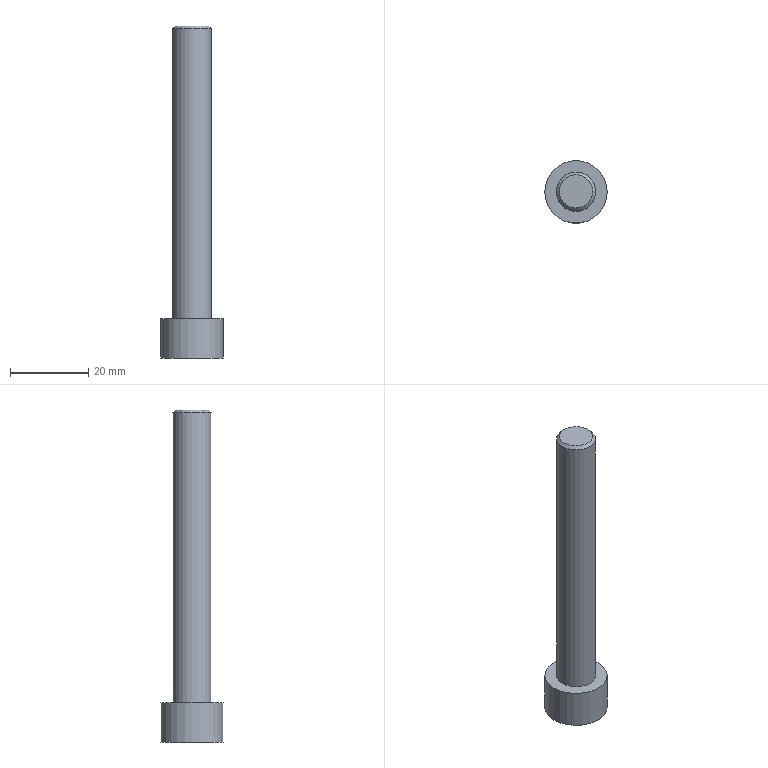Part | STEP file | gslz 2016.10.28-6_id290_x_t | 1 solid | 13 faces | box 16 x 16 x 85 mm | volume 7560 mm3 | plane 10 | cylinder 2 | cone 1 | commonest cylinder face diameters 10 x1 16 x1
STEP:
#1=CARTESIAN_POINT('',(-19.95,98.309,66.992));
#2=VERTEX_POINT('',#1);
#3=CARTESIAN_POINT('',(-19.95,93.691,66.992));
#4=VERTEX_POINT('',#3);
#5=CARTESIAN_POINT('',(-19.95,98.309,66.992));
#6=DIRECTION('',(0.,-1.,0.));
#7=VECTOR('',#6,1.);
#8=LINE('',#5,#7);
#9=EDGE_CURVE('',#2,#4,#8,.T.);
#10=ORIENTED_EDGE('',*,*,#9,.T.);
#11=CARTESIAN_POINT('',(-15.95,91.381,66.992));
#12=VERTEX_POINT('',#11);
#13=CARTESIAN_POINT('',(-19.95,93.691,66.992));
#14=DIRECTION('',(0.866,-0.5,0.));
#15=VECTOR('',#14,1.);
#16=LINE('',#13,#15);
#17=EDGE_CURVE('',#4,#12,#16,.T.);
#18=ORIENTED_EDGE('',*,*,#17,.T.);
#19=CARTESIAN_POINT('',(-11.95,93.691,66.992));
#20=VERTEX_POINT('',#19);
#21=CARTESIAN_POINT('',(-15.95,91.381,66.992));
#22=DIRECTION('',(0.866,0.5,0.));
#23=VECTOR('',#22,1.);
#24=LINE('',#21,#23);
#25=EDGE_CURVE('',#12,#20,#24,.T.);
#26=ORIENTED_EDGE('',*,*,#25,.T.);
#27=CARTESIAN_POINT('',(-11.95,98.309,66.992));
#28=VERTEX_POINT('',#27);
#29=CARTESIAN_POINT('',(-11.95,93.691,66.992));
#30=DIRECTION('',(0.,1.,0.));
#31=VECTOR('',#30,1.);
#32=LINE('',#29,#31);
#33=EDGE_CURVE('',#20,#28,#32,.T.);
#34=ORIENTED_EDGE('',*,*,#33,.T.);
#35=CARTESIAN_POINT('',(-15.95,100.619,66.992));
#36=VERTEX_POINT('',#35);
#37=CARTESIAN_POINT('',(-11.95,98.309,66.992));
#38=DIRECTION('',(-0.866,0.5,0.));
#39=VECTOR('',#38,1.);
#40=LINE('',#37,#39);
#41=EDGE_CURVE('',#28,#36,#40,.T.);
#42=ORIENTED_EDGE('',*,*,#41,.T.);
#43=CARTESIAN_POINT('',(-15.95,100.619,66.992));
#44=DIRECTION('',(-0.866,-0.5,0.));
#45=VECTOR('',#44,1.);
#46=LINE('',#43,#45);
#47=EDGE_CURVE('',#36,#2,#46,.T.);
#48=ORIENTED_EDGE('',*,*,#47,.T.);
#49=EDGE_LOOP('',(#10,#18,#26,#34,#42,#48));
#50=FACE_BOUND('',#49,.T.);
#51=CARTESIAN_POINT('',(-7.95,96.,66.992));
#52=VERTEX_POINT('',#51);
#53=CARTESIAN_POINT('',(-15.95,96.,66.992));
#54=DIRECTION('',(0.,0.,-1.));
#55=DIRECTION('',(1.,0.,0.));
#56=AXIS2_PLACEMENT_3D('',#53,#54,#55);
#57=CIRCLE('',#56,8.);
#58=EDGE_CURVE('',#52,#52,#57,.T.);
#59=ORIENTED_EDGE('',*,*,#58,.T.);
#60=EDGE_LOOP('',(#59));
#61=FACE_BOUND('',#60,.T.);
#62=CARTESIAN_POINT('',(-15.95,96.,66.992));
#63=DIRECTION('',(0.,0.,-1.));
#64=DIRECTION('',(-1.,0.,0.));
#65=AXIS2_PLACEMENT_3D('',#62,#63,#64);
#66=PLANE('',#65);
#67=ADVANCED_FACE('',(#50,#61),#66,.T.);
#68=CARTESIAN_POINT('',(-20.2,96.,151.992));
#69=VERTEX_POINT('',#68);
#70=CARTESIAN_POINT('',(-15.95,96.,151.992));
#71=DIRECTION('',(0.,0.,-1.));
#72=DIRECTION('',(-1.,0.,0.));
#73=AXIS2_PLACEMENT_3D('',#70,#71,#72);
#74=CIRCLE('',#73,4.25);
#75=EDGE_CURVE('',#69,#69,#74,.T.);
#76=ORIENTED_EDGE('',*,*,#75,.F.);
#77=EDGE_LOOP('',(#76));
#78=FACE_OUTER_BOUND('',#77,.T.);
#79=CARTESIAN_POINT('',(-15.95,96.,151.992));
#80=DIRECTION('',(0.,0.,1.));
#81=DIRECTION('',(1.,0.,0.));
#82=AXIS2_PLACEMENT_3D('',#79,#80,#81);
#83=PLANE('',#82);
#84=ADVANCED_FACE('',(#78),#83,.T.);
#85=CARTESIAN_POINT('',(-20.95,96.,151.242));
#86=VERTEX_POINT('',#85);
#87=CARTESIAN_POINT('',(-15.95,96.,151.242));
#88=DIRECTION('',(0.,0.,1.));
#89=DIRECTION('',(-1.,0.,0.));
#90=AXIS2_PLACEMENT_3D('',#87,#88,#89);
#91=CIRCLE('',#90,5.);
#92=EDGE_CURVE('',#86,#86,#91,.T.);
#93=ORIENTED_EDGE('',*,*,#92,.F.);
#94=EDGE_LOOP('',(#93));
#95=FACE_BOUND('',#94,.T.);
#96=CARTESIAN_POINT('',(-20.95,96.,76.992));
#97=VERTEX_POINT('',#96);
#98=CARTESIAN_POINT('',(-15.95,96.,76.992));
#99=DIRECTION('',(0.,0.,-1.));
#100=DIRECTION('',(-1.,0.,0.));
#101=AXIS2_PLACEMENT_3D('',#98,#99,#100);
#102=CIRCLE('',#101,5.);
#103=EDGE_CURVE('',#97,#97,#102,.T.);
#104=ORIENTED_EDGE('',*,*,#103,.F.);
#105=EDGE_LOOP('',(#104));
#106=FACE_BOUND('',#105,.T.);
#107=CARTESIAN_POINT('',(-15.95,96.,96.992));
#108=DIRECTION('',(0.,0.,1.));
#109=DIRECTION('',(1.,0.,0.));
#110=AXIS2_PLACEMENT_3D('',#107,#108,#109);
#111=CYLINDRICAL_SURFACE('',#110,5.);
#112=ADVANCED_FACE('',(#95,#106),#111,.T.);
#113=ORIENTED_EDGE('',*,*,#103,.T.);
#114=EDGE_LOOP('',(#113));
#115=FACE_BOUND('',#114,.T.);
#116=CARTESIAN_POINT('',(-23.95,96.,76.992));
#117=VERTEX_POINT('',#116);
#118=CARTESIAN_POINT('',(-15.95,96.,76.992));
#119=DIRECTION('',(0.,0.,-1.));
#120=DIRECTION('',(-1.,0.,0.));
#121=AXIS2_PLACEMENT_3D('',#118,#119,#120);
#122=CIRCLE('',#121,8.);
#123=EDGE_CURVE('',#117,#117,#122,.T.);
#124=ORIENTED_EDGE('',*,*,#123,.F.);
#125=EDGE_LOOP('',(#124));
#126=FACE_BOUND('',#125,.T.);
#127=CARTESIAN_POINT('',(-15.95,96.,76.992));
#128=DIRECTION('',(0.,0.,1.));
#129=DIRECTION('',(1.,0.,0.));
#130=AXIS2_PLACEMENT_3D('',#127,#128,#129);
#131=PLANE('',#130);
#132=ADVANCED_FACE('',(#115,#126),#131,.T.);
#133=ORIENTED_EDGE('',*,*,#123,.T.);
#134=EDGE_LOOP('',(#133));
#135=FACE_BOUND('',#134,.T.);
#136=ORIENTED_EDGE('',*,*,#58,.F.);
#137=EDGE_LOOP('',(#136));
#138=FACE_BOUND('',#137,.T.);
#139=CARTESIAN_POINT('',(-15.95,96.,63.992));
#140=DIRECTION('',(0.,0.,1.));
#141=DIRECTION('',(1.,0.,0.));
#142=AXIS2_PLACEMENT_3D('',#139,#140,#141);
#143=CYLINDRICAL_SURFACE('',#142,8.);
#144=ADVANCED_FACE('',(#135,#138),#143,.T.);
#145=ORIENTED_EDGE('',*,*,#9,.F.);
#146=CARTESIAN_POINT('',(-19.95,98.309,72.992));
#147=VERTEX_POINT('',#146);
#148=CARTESIAN_POINT('',(-19.95,98.309,72.992));
#149=DIRECTION('',(0.,0.,1.));
#150=VECTOR('',#149,1.);
#151=LINE('',#148,#150);
#152=EDGE_CURVE('',#2,#147,#151,.T.);
#153=ORIENTED_EDGE('',*,*,#152,.T.);
#154=CARTESIAN_POINT('',(-19.95,93.691,72.992));
#155=VERTEX_POINT('',#154);
#156=CARTESIAN_POINT('',(-19.95,98.309,72.992));
#157=DIRECTION('',(0.,1.,0.));
#158=VECTOR('',#157,1.);
#159=LINE('',#156,#158);
#160=EDGE_CURVE('',#155,#147,#159,.T.);
#161=ORIENTED_EDGE('',*,*,#160,.F.);
#162=CARTESIAN_POINT('',(-19.95,93.691,72.992));
#163=DIRECTION('',(0.,0.,1.));
#164=VECTOR('',#163,1.);
#165=LINE('',#162,#164);
#166=EDGE_CURVE('',#4,#155,#165,.T.);
#167=ORIENTED_EDGE('',*,*,#166,.F.);
#168=EDGE_LOOP('',(#145,#153,#161,#167));
#169=FACE_OUTER_BOUND('',#168,.T.);
#170=CARTESIAN_POINT('',(-19.95,98.309,72.992));
#171=DIRECTION('',(-1.,0.,0.));
#172=DIRECTION('',(0.,0.,1.));
#173=AXIS2_PLACEMENT_3D('',#170,#171,#172);
#174=PLANE('',#173);
#175=ADVANCED_FACE('',(#169),#174,.F.);
#176=ORIENTED_EDGE('',*,*,#17,.F.);
#177=ORIENTED_EDGE('',*,*,#166,.T.);
#178=CARTESIAN_POINT('',(-15.95,91.381,72.992));
#179=VERTEX_POINT('',#178);
#180=CARTESIAN_POINT('',(-19.95,93.691,72.992));
#181=DIRECTION('',(-0.866,0.5,0.));
#182=VECTOR('',#181,1.);
#183=LINE('',#180,#182);
#184=EDGE_CURVE('',#179,#155,#183,.T.);
#185=ORIENTED_EDGE('',*,*,#184,.F.);
#186=CARTESIAN_POINT('',(-15.95,91.381,72.992));
#187=DIRECTION('',(0.,0.,1.));
#188=VECTOR('',#187,1.);
#189=LINE('',#186,#188);
#190=EDGE_CURVE('',#12,#179,#189,.T.);
#191=ORIENTED_EDGE('',*,*,#190,.F.);
#192=EDGE_LOOP('',(#176,#177,#185,#191));
#193=FACE_OUTER_BOUND('',#192,.T.);
#194=CARTESIAN_POINT('',(-19.95,93.691,72.992));
#195=DIRECTION('',(-0.5,-0.866,0.));
#196=DIRECTION('',(-0.866,0.5,0.));
#197=AXIS2_PLACEMENT_3D('',#194,#195,#196);
#198=PLANE('',#197);
#199=ADVANCED_FACE('',(#193),#198,.F.);
#200=ORIENTED_EDGE('',*,*,#25,.F.);
#201=ORIENTED_EDGE('',*,*,#190,.T.);
#202=CARTESIAN_POINT('',(-11.95,93.691,72.992));
#203=VERTEX_POINT('',#202);
#204=CARTESIAN_POINT('',(-15.95,91.381,72.992));
#205=DIRECTION('',(-0.866,-0.5,0.));
#206=VECTOR('',#205,1.);
#207=LINE('',#204,#206);
#208=EDGE_CURVE('',#203,#179,#207,.T.);
#209=ORIENTED_EDGE('',*,*,#208,.F.);
#210=CARTESIAN_POINT('',(-11.95,93.691,72.992));
#211=DIRECTION('',(0.,0.,1.));
#212=VECTOR('',#211,1.);
#213=LINE('',#210,#212);
#214=EDGE_CURVE('',#20,#203,#213,.T.);
#215=ORIENTED_EDGE('',*,*,#214,.F.);
#216=EDGE_LOOP('',(#200,#201,#209,#215));
#217=FACE_OUTER_BOUND('',#216,.T.);
#218=CARTESIAN_POINT('',(-15.95,91.381,72.992));
#219=DIRECTION('',(0.5,-0.866,0.));
#220=DIRECTION('',(-0.866,-0.5,0.));
#221=AXIS2_PLACEMENT_3D('',#218,#219,#220);
#222=PLANE('',#221);
#223=ADVANCED_FACE('',(#217),#222,.F.);
#224=ORIENTED_EDGE('',*,*,#33,.F.);
#225=ORIENTED_EDGE('',*,*,#214,.T.);
#226=CARTESIAN_POINT('',(-11.95,98.309,72.992));
#227=VERTEX_POINT('',#226);
#228=CARTESIAN_POINT('',(-11.95,93.691,72.992));
#229=DIRECTION('',(0.,-1.,0.));
#230=VECTOR('',#229,1.);
#231=LINE('',#228,#230);
#232=EDGE_CURVE('',#227,#203,#231,.T.);
#233=ORIENTED_EDGE('',*,*,#232,.F.);
#234=CARTESIAN_POINT('',(-11.95,98.309,72.992));
#235=DIRECTION('',(0.,0.,1.));
#236=VECTOR('',#235,1.);
#237=LINE('',#234,#236);
#238=EDGE_CURVE('',#28,#227,#237,.T.);
#239=ORIENTED_EDGE('',*,*,#238,.F.);
#240=EDGE_LOOP('',(#224,#225,#233,#239));
#241=FACE_OUTER_BOUND('',#240,.T.);
#242=CARTESIAN_POINT('',(-11.95,93.691,72.992));
#243=DIRECTION('',(1.,0.,0.));
#244=DIRECTION('',(0.,0.,-1.));
#245=AXIS2_PLACEMENT_3D('',#242,#243,#244);
#246=PLANE('',#245);
#247=ADVANCED_FACE('',(#241),#246,.F.);
#248=ORIENTED_EDGE('',*,*,#41,.F.);
#249=ORIENTED_EDGE('',*,*,#238,.T.);
#250=CARTESIAN_POINT('',(-15.95,100.619,72.992));
#251=VERTEX_POINT('',#250);
#252=CARTESIAN_POINT('',(-11.95,98.309,72.992));
#253=DIRECTION('',(0.866,-0.5,0.));
#254=VECTOR('',#253,1.);
#255=LINE('',#252,#254);
#256=EDGE_CURVE('',#251,#227,#255,.T.);
#257=ORIENTED_EDGE('',*,*,#256,.F.);
#258=CARTESIAN_POINT('',(-15.95,100.619,72.992));
#259=DIRECTION('',(0.,0.,1.));
#260=VECTOR('',#259,1.);
#261=LINE('',#258,#260);
#262=EDGE_CURVE('',#36,#251,#261,.T.);
#263=ORIENTED_EDGE('',*,*,#262,.F.);
#264=EDGE_LOOP('',(#248,#249,#257,#263));
#265=FACE_OUTER_BOUND('',#264,.T.);
#266=CARTESIAN_POINT('',(-11.95,98.309,72.992));
#267=DIRECTION('',(0.5,0.866,0.));
#268=DIRECTION('',(0.866,-0.5,0.));
#269=AXIS2_PLACEMENT_3D('',#266,#267,#268);
#270=PLANE('',#269);
#271=ADVANCED_FACE('',(#265),#270,.F.);
#272=ORIENTED_EDGE('',*,*,#47,.F.);
#273=ORIENTED_EDGE('',*,*,#262,.T.);
#274=CARTESIAN_POINT('',(-15.95,100.619,72.992));
#275=DIRECTION('',(0.866,0.5,0.));
#276=VECTOR('',#275,1.);
#277=LINE('',#274,#276);
#278=EDGE_CURVE('',#147,#251,#277,.T.);
#279=ORIENTED_EDGE('',*,*,#278,.F.);
#280=ORIENTED_EDGE('',*,*,#152,.F.);
#281=EDGE_LOOP('',(#272,#273,#279,#280));
#282=FACE_OUTER_BOUND('',#281,.T.);
#283=CARTESIAN_POINT('',(-15.95,100.619,72.992));
#284=DIRECTION('',(-0.5,0.866,0.));
#285=DIRECTION('',(0.866,0.5,0.));
#286=AXIS2_PLACEMENT_3D('',#283,#284,#285);
#287=PLANE('',#286);
#288=ADVANCED_FACE('',(#282),#287,.F.);
#289=ORIENTED_EDGE('',*,*,#160,.T.);
#290=ORIENTED_EDGE('',*,*,#278,.T.);
#291=ORIENTED_EDGE('',*,*,#256,.T.);
#292=ORIENTED_EDGE('',*,*,#232,.T.);
#293=ORIENTED_EDGE('',*,*,#208,.T.);
#294=ORIENTED_EDGE('',*,*,#184,.T.);
#295=EDGE_LOOP('',(#289,#290,#291,#292,#293,#294));
#296=FACE_OUTER_BOUND('',#295,.T.);
#297=CARTESIAN_POINT('',(-19.95,93.691,72.992));
#298=DIRECTION('',(0.,0.,-1.));
#299=DIRECTION('',(-1.,0.,0.));
#300=AXIS2_PLACEMENT_3D('',#297,#298,#299);
#301=PLANE('',#300);
#302=ADVANCED_FACE('',(#296),#301,.T.);
#303=ORIENTED_EDGE('',*,*,#92,.T.);
#304=EDGE_LOOP('',(#303));
#305=FACE_BOUND('',#304,.T.);
#306=ORIENTED_EDGE('',*,*,#75,.T.);
#307=EDGE_LOOP('',(#306));
#308=FACE_BOUND('',#307,.T.);
#309=CARTESIAN_POINT('',(-15.95,96.,151.992));
#310=DIRECTION('',(0.,0.,-1.));
#311=DIRECTION('',(-1.,0.,0.));
#312=AXIS2_PLACEMENT_3D('',#309,#310,#311);
#313=CONICAL_SURFACE('',#312,4.25,45.);
#314=ADVANCED_FACE('',(#305,#308),#313,.T.);
#315=CLOSED_SHELL('',(#67,#84,#112,#132,#144,#175,#199,#223,#247,#271,#288,#302,#314));
#316=MANIFOLD_SOLID_BREP('',#315);
#317=(LENGTH_UNIT()NAMED_UNIT(*)SI_UNIT(.MILLI.,.METRE.));
#318=UNCERTAINTY_MEASURE_WITH_UNIT(LENGTH_MEASURE(0.00002),#317,'','');
#319=(NAMED_UNIT(*)PLANE_ANGLE_UNIT()SI_UNIT($,.RADIAN.));
#320=PLANE_ANGLE_MEASURE_WITH_UNIT(PLANE_ANGLE_MEASURE(0.01745),#319);
#321=DIMENSIONAL_EXPONENTS(0.,0.,0.,0.,0.,0.,0.);
#322=(CONVERSION_BASED_UNIT('DEGREE',#320)NAMED_UNIT(#321)PLANE_ANGLE_UNIT());
#323=(NAMED_UNIT(*)SI_UNIT($,.STERADIAN.)SOLID_ANGLE_UNIT());
#324=(GEOMETRIC_REPRESENTATION_CONTEXT(3)GLOBAL_UNCERTAINTY_ASSIGNED_CONTEXT((#318))GLOBAL_UNIT_ASSIGNED_CONTEXT((#317,#322,#323))REPRESENTATION_CONTEXT('',''));
#325=ADVANCED_BREP_SHAPE_REPRESENTATION('',(#316),#324);